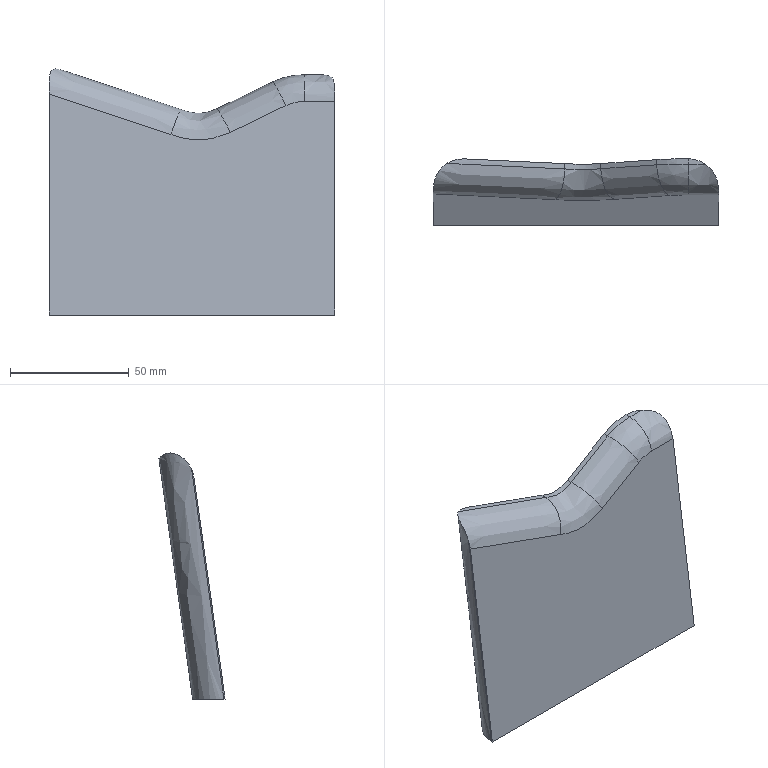Part | STEP file | solid 56 | 1 solid | 17 faces | box 120 x 27.824 x 103.411 mm | volume 144143 mm3 | spline 9 | other 5 | plane 3